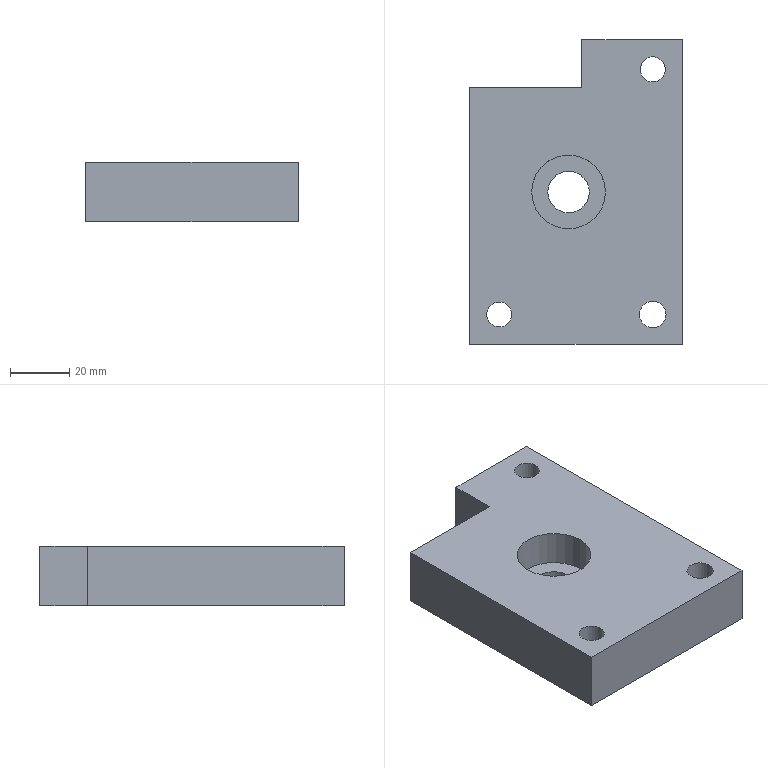Part | NX | features solid 2 | 1 solid | 20 faces | box 72 x 103 x 20 mm | volume 122631 mm3 | plane 12 | cylinder 8 | commonest cylinder face diameters 14 x3 8.5 x2 9 x1 14.1 x1 25 x1
STEP:
#1=CARTESIAN_POINT('',(121.25,98.5,20.));
#2=VERTEX_POINT('',#1);
#3=CARTESIAN_POINT('',(125.5,98.5,20.));
#4=DIRECTION('',(0.,0.,-1.));
#5=DIRECTION('',(-1.,0.,0.));
#6=AXIS2_PLACEMENT_3D('',#3,#4,#5);
#7=CIRCLE('',#6,4.25);
#8=EDGE_CURVE('',#2,#2,#7,.T.);
#9=ORIENTED_EDGE('',*,*,#8,.F.);
#10=EDGE_LOOP('',(#9));
#11=FACE_BOUND('',#10,.T.);
#12=CARTESIAN_POINT('',(121.25,98.5,10.));
#13=VERTEX_POINT('',#12);
#14=CARTESIAN_POINT('',(125.5,98.5,10.));
#15=DIRECTION('',(0.,0.,-1.));
#16=DIRECTION('',(-1.,0.,0.));
#17=AXIS2_PLACEMENT_3D('',#14,#15,#16);
#18=CIRCLE('',#17,4.25);
#19=EDGE_CURVE('',#13,#13,#18,.T.);
#20=ORIENTED_EDGE('',*,*,#19,.T.);
#21=EDGE_LOOP('',(#20));
#22=FACE_BOUND('',#21,.T.);
#23=CARTESIAN_POINT('',(125.5,98.5,35.));
#24=DIRECTION('',(0.,0.,1.));
#25=DIRECTION('',(1.,0.,0.));
#26=AXIS2_PLACEMENT_3D('',#23,#24,#25);
#27=CYLINDRICAL_SURFACE('',#26,4.25);
#28=ADVANCED_FACE('',(#11,#22),#27,.F.);
#29=CARTESIAN_POINT('',(118.5,98.5,10.));
#30=VERTEX_POINT('',#29);
#31=CARTESIAN_POINT('',(125.5,98.5,10.));
#32=DIRECTION('',(0.,0.,-1.));
#33=DIRECTION('',(-1.,0.,0.));
#34=AXIS2_PLACEMENT_3D('',#31,#32,#33);
#35=CIRCLE('',#34,7.);
#36=EDGE_CURVE('',#30,#30,#35,.T.);
#37=ORIENTED_EDGE('',*,*,#36,.F.);
#38=EDGE_LOOP('',(#37));
#39=FACE_BOUND('',#38,.T.);
#40=CARTESIAN_POINT('',(132.5,98.5,0.00000121));
#41=VERTEX_POINT('',#40);
#42=CARTESIAN_POINT('',(125.5,98.5,0.00000121));
#43=DIRECTION('',(0.,0.,1.));
#44=DIRECTION('',(1.,0.,0.));
#45=AXIS2_PLACEMENT_3D('',#42,#43,#44);
#46=CIRCLE('',#45,7.);
#47=EDGE_CURVE('',#41,#41,#46,.T.);
#48=ORIENTED_EDGE('',*,*,#47,.F.);
#49=EDGE_LOOP('',(#48));
#50=FACE_BOUND('',#49,.T.);
#51=CARTESIAN_POINT('',(125.5,98.5,0.00000121));
#52=DIRECTION('',(0.,0.,1.));
#53=DIRECTION('',(1.,0.,0.));
#54=AXIS2_PLACEMENT_3D('',#51,#52,#53);
#55=CYLINDRICAL_SURFACE('',#54,7.);
#56=ADVANCED_FACE('',(#39,#50),#55,.F.);
#57=ORIENTED_EDGE('',*,*,#19,.F.);
#58=EDGE_LOOP('',(#57));
#59=FACE_BOUND('',#58,.T.);
#60=ORIENTED_EDGE('',*,*,#36,.T.);
#61=EDGE_LOOP('',(#60));
#62=FACE_BOUND('',#61,.T.);
#63=CARTESIAN_POINT('',(11.595,84.569,10.));
#64=DIRECTION('',(0.,0.,1.));
#65=DIRECTION('',(-1.,0.,0.));
#66=AXIS2_PLACEMENT_3D('',#63,#64,#65);
#67=PLANE('',#66);
#68=ADVANCED_FACE('',(#59,#62),#67,.F.);
#69=CARTESIAN_POINT('',(182.,98.5,10.));
#70=VERTEX_POINT('',#69);
#71=CARTESIAN_POINT('',(177.5,98.5,10.));
#72=DIRECTION('',(0.,0.,1.));
#73=DIRECTION('',(1.,0.,0.));
#74=AXIS2_PLACEMENT_3D('',#71,#72,#73);
#75=CIRCLE('',#74,4.5);
#76=EDGE_CURVE('',#70,#70,#75,.F.);
#77=ORIENTED_EDGE('',*,*,#76,.F.);
#78=EDGE_LOOP('',(#77));
#79=FACE_BOUND('',#78,.T.);
#80=CARTESIAN_POINT('',(184.5,98.5,10.));
#81=VERTEX_POINT('',#80);
#82=CARTESIAN_POINT('',(177.5,98.5,10.));
#83=DIRECTION('',(0.,0.,1.));
#84=DIRECTION('',(1.,0.,0.));
#85=AXIS2_PLACEMENT_3D('',#82,#83,#84);
#86=CIRCLE('',#85,7.);
#87=EDGE_CURVE('',#81,#81,#86,.F.);
#88=ORIENTED_EDGE('',*,*,#87,.T.);
#89=EDGE_LOOP('',(#88));
#90=FACE_BOUND('',#89,.T.);
#91=CARTESIAN_POINT('',(291.405,84.569,10.));
#92=DIRECTION('',(0.,0.,1.));
#93=DIRECTION('',(1.,0.,0.));
#94=AXIS2_PLACEMENT_3D('',#91,#92,#93);
#95=PLANE('',#94);
#96=ADVANCED_FACE('',(#79,#90),#95,.F.);
#97=CARTESIAN_POINT('',(181.75,181.5,10.));
#98=VERTEX_POINT('',#97);
#99=CARTESIAN_POINT('',(177.5,181.5,10.));
#100=DIRECTION('',(0.,0.,-1.));
#101=DIRECTION('',(1.,0.,0.));
#102=AXIS2_PLACEMENT_3D('',#99,#100,#101);
#103=CIRCLE('',#102,4.25);
#104=EDGE_CURVE('',#98,#98,#103,.T.);
#105=ORIENTED_EDGE('',*,*,#104,.F.);
#106=EDGE_LOOP('',(#105));
#107=FACE_BOUND('',#106,.T.);
#108=CARTESIAN_POINT('',(184.5,181.5,10.));
#109=VERTEX_POINT('',#108);
#110=CARTESIAN_POINT('',(177.5,181.5,10.));
#111=DIRECTION('',(0.,0.,-1.));
#112=DIRECTION('',(1.,0.,0.));
#113=AXIS2_PLACEMENT_3D('',#110,#111,#112);
#114=CIRCLE('',#113,7.);
#115=EDGE_CURVE('',#109,#109,#114,.T.);
#116=ORIENTED_EDGE('',*,*,#115,.T.);
#117=EDGE_LOOP('',(#116));
#118=FACE_BOUND('',#117,.T.);
#119=CARTESIAN_POINT('',(291.405,195.431,10.));
#120=DIRECTION('',(0.,0.,1.));
#121=DIRECTION('',(1.,0.,0.));
#122=AXIS2_PLACEMENT_3D('',#119,#120,#121);
#123=PLANE('',#122);
#124=ADVANCED_FACE('',(#107,#118),#123,.F.);
#125=ORIENTED_EDGE('',*,*,#87,.F.);
#126=EDGE_LOOP('',(#125));
#127=FACE_BOUND('',#126,.T.);
#128=CARTESIAN_POINT('',(170.5,98.5,0.00000121));
#129=VERTEX_POINT('',#128);
#130=CARTESIAN_POINT('',(177.5,98.5,0.00000121));
#131=DIRECTION('',(0.,0.,-1.));
#132=DIRECTION('',(-1.,0.,0.));
#133=AXIS2_PLACEMENT_3D('',#130,#131,#132);
#134=CIRCLE('',#133,7.);
#135=EDGE_CURVE('',#129,#129,#134,.F.);
#136=ORIENTED_EDGE('',*,*,#135,.F.);
#137=EDGE_LOOP('',(#136));
#138=FACE_BOUND('',#137,.T.);
#139=CARTESIAN_POINT('',(177.5,98.5,0.00000121));
#140=DIRECTION('',(0.,0.,1.));
#141=DIRECTION('',(-1.,0.,0.));
#142=AXIS2_PLACEMENT_3D('',#139,#140,#141);
#143=CYLINDRICAL_SURFACE('',#142,7.);
#144=ADVANCED_FACE('',(#127,#138),#143,.F.);
#145=ORIENTED_EDGE('',*,*,#115,.F.);
#146=EDGE_LOOP('',(#145));
#147=FACE_BOUND('',#146,.T.);
#148=CARTESIAN_POINT('',(170.5,181.5,0.00000121));
#149=VERTEX_POINT('',#148);
#150=CARTESIAN_POINT('',(177.5,181.5,0.00000121));
#151=DIRECTION('',(0.,0.,1.));
#152=DIRECTION('',(-1.,0.,0.));
#153=AXIS2_PLACEMENT_3D('',#150,#151,#152);
#154=CIRCLE('',#153,7.);
#155=EDGE_CURVE('',#149,#149,#154,.T.);
#156=ORIENTED_EDGE('',*,*,#155,.F.);
#157=EDGE_LOOP('',(#156));
#158=FACE_BOUND('',#157,.T.);
#159=CARTESIAN_POINT('',(177.5,181.5,0.00000121));
#160=DIRECTION('',(0.,0.,1.));
#161=DIRECTION('',(-1.,0.,0.));
#162=AXIS2_PLACEMENT_3D('',#159,#160,#161);
#163=CYLINDRICAL_SURFACE('',#162,7.);
#164=ADVANCED_FACE('',(#147,#158),#163,.F.);
#165=CARTESIAN_POINT('',(161.5,140.,8.));
#166=VERTEX_POINT('',#165);
#167=CARTESIAN_POINT('',(149.,140.,8.));
#168=DIRECTION('',(0.,0.,1.));
#169=DIRECTION('',(1.,0.,0.));
#170=AXIS2_PLACEMENT_3D('',#167,#168,#169);
#171=CIRCLE('',#170,12.5);
#172=EDGE_CURVE('',#166,#166,#171,.F.);
#173=ORIENTED_EDGE('',*,*,#172,.T.);
#174=EDGE_LOOP('',(#173));
#175=FACE_BOUND('',#174,.T.);
#176=CARTESIAN_POINT('',(161.5,140.,20.));
#177=VERTEX_POINT('',#176);
#178=CARTESIAN_POINT('',(149.,140.,20.));
#179=DIRECTION('',(0.,0.,1.));
#180=DIRECTION('',(1.,0.,0.));
#181=AXIS2_PLACEMENT_3D('',#178,#179,#180);
#182=CIRCLE('',#181,12.5);
#183=EDGE_CURVE('',#177,#177,#182,.F.);
#184=ORIENTED_EDGE('',*,*,#183,.F.);
#185=EDGE_LOOP('',(#184));
#186=FACE_BOUND('',#185,.T.);
#187=CARTESIAN_POINT('',(149.,140.,2.5));
#188=DIRECTION('',(0.,0.,-1.));
#189=DIRECTION('',(-1.,0.,0.));
#190=AXIS2_PLACEMENT_3D('',#187,#188,#189);
#191=CYLINDRICAL_SURFACE('',#190,12.5);
#192=ADVANCED_FACE('',(#175,#186),#191,.F.);
#193=CARTESIAN_POINT('',(187.5,88.5,20.));
#194=VERTEX_POINT('',#193);
#195=CARTESIAN_POINT('',(187.5,88.5,0.00000121));
#196=VERTEX_POINT('',#195);
#197=CARTESIAN_POINT('',(187.5,88.5,35.));
#198=DIRECTION('',(0.,0.,-1.));
#199=VECTOR('',#198,1000.);
#200=LINE('',#197,#199);
#201=EDGE_CURVE('',#194,#196,#200,.T.);
#202=ORIENTED_EDGE('',*,*,#201,.T.);
#203=CARTESIAN_POINT('',(187.5,191.5,0.00000121));
#204=VERTEX_POINT('',#203);
#205=CARTESIAN_POINT('',(187.5,140.,0.00000121));
#206=DIRECTION('',(0.,-1.,0.));
#207=VECTOR('',#206,1000.);
#208=LINE('',#205,#207);
#209=EDGE_CURVE('',#196,#204,#208,.F.);
#210=ORIENTED_EDGE('',*,*,#209,.T.);
#211=CARTESIAN_POINT('',(187.5,191.5,20.));
#212=VERTEX_POINT('',#211);
#213=CARTESIAN_POINT('',(187.5,191.5,35.));
#214=DIRECTION('',(0.,0.,-1.));
#215=VECTOR('',#214,1000.);
#216=LINE('',#213,#215);
#217=EDGE_CURVE('',#212,#204,#216,.T.);
#218=ORIENTED_EDGE('',*,*,#217,.F.);
#219=CARTESIAN_POINT('',(187.5,140.,20.));
#220=DIRECTION('',(0.,1.,0.));
#221=VECTOR('',#220,1000.);
#222=LINE('',#219,#221);
#223=EDGE_CURVE('',#194,#212,#222,.T.);
#224=ORIENTED_EDGE('',*,*,#223,.F.);
#225=EDGE_LOOP('',(#202,#210,#218,#224));
#226=FACE_BOUND('',#225,.T.);
#227=CARTESIAN_POINT('',(187.5,140.,35.));
#228=DIRECTION('',(-1.,0.,0.));
#229=DIRECTION('',(0.,1.,0.));
#230=AXIS2_PLACEMENT_3D('',#227,#228,#229);
#231=PLANE('',#230);
#232=ADVANCED_FACE('',(#226),#231,.F.);
#233=CARTESIAN_POINT('',(115.5,88.5,20.));
#234=VERTEX_POINT('',#233);
#235=CARTESIAN_POINT('',(115.5,88.5,0.00000121));
#236=VERTEX_POINT('',#235);
#237=CARTESIAN_POINT('',(115.5,88.5,35.));
#238=DIRECTION('',(0.,0.,-1.));
#239=VECTOR('',#238,1000.);
#240=LINE('',#237,#239);
#241=EDGE_CURVE('',#234,#236,#240,.T.);
#242=ORIENTED_EDGE('',*,*,#241,.T.);
#243=CARTESIAN_POINT('',(149.,88.5,0.00000121));
#244=DIRECTION('',(-1.,0.,0.));
#245=VECTOR('',#244,1000.);
#246=LINE('',#243,#245);
#247=EDGE_CURVE('',#236,#196,#246,.F.);
#248=ORIENTED_EDGE('',*,*,#247,.T.);
#249=ORIENTED_EDGE('',*,*,#201,.F.);
#250=CARTESIAN_POINT('',(149.,88.5,20.));
#251=DIRECTION('',(1.,0.,0.));
#252=VECTOR('',#251,1000.);
#253=LINE('',#250,#252);
#254=EDGE_CURVE('',#234,#194,#253,.T.);
#255=ORIENTED_EDGE('',*,*,#254,.F.);
#256=EDGE_LOOP('',(#242,#248,#249,#255));
#257=FACE_BOUND('',#256,.T.);
#258=CARTESIAN_POINT('',(149.,88.5,35.));
#259=DIRECTION('',(0.,1.,0.));
#260=DIRECTION('',(1.,0.,0.));
#261=AXIS2_PLACEMENT_3D('',#258,#259,#260);
#262=PLANE('',#261);
#263=ADVANCED_FACE('',(#257),#262,.F.);
#264=CARTESIAN_POINT('',(115.5,175.5,0.00000121));
#265=VERTEX_POINT('',#264);
#266=CARTESIAN_POINT('',(115.5,175.5,20.));
#267=VERTEX_POINT('',#266);
#268=CARTESIAN_POINT('',(115.5,175.5,35.));
#269=DIRECTION('',(0.,0.,1.));
#270=VECTOR('',#269,1000.);
#271=LINE('',#268,#270);
#272=EDGE_CURVE('',#265,#267,#271,.T.);
#273=ORIENTED_EDGE('',*,*,#272,.F.);
#274=CARTESIAN_POINT('',(115.5,140.,0.00000121));
#275=DIRECTION('',(0.,1.,0.));
#276=VECTOR('',#275,1000.);
#277=LINE('',#274,#276);
#278=EDGE_CURVE('',#265,#236,#277,.F.);
#279=ORIENTED_EDGE('',*,*,#278,.T.);
#280=ORIENTED_EDGE('',*,*,#241,.F.);
#281=CARTESIAN_POINT('',(115.5,140.,20.));
#282=DIRECTION('',(0.,-1.,0.));
#283=VECTOR('',#282,1000.);
#284=LINE('',#281,#283);
#285=EDGE_CURVE('',#267,#234,#284,.T.);
#286=ORIENTED_EDGE('',*,*,#285,.F.);
#287=EDGE_LOOP('',(#273,#279,#280,#286));
#288=FACE_BOUND('',#287,.T.);
#289=CARTESIAN_POINT('',(115.5,140.,35.));
#290=DIRECTION('',(1.,0.,0.));
#291=DIRECTION('',(0.,-1.,0.));
#292=AXIS2_PLACEMENT_3D('',#289,#290,#291);
#293=PLANE('',#292);
#294=ADVANCED_FACE('',(#288),#293,.F.);
#295=CARTESIAN_POINT('',(153.5,175.5,20.));
#296=VERTEX_POINT('',#295);
#297=CARTESIAN_POINT('',(153.5,175.5,0.00000121));
#298=VERTEX_POINT('',#297);
#299=CARTESIAN_POINT('',(153.5,175.5,-10.));
#300=DIRECTION('',(0.,0.,1.));
#301=VECTOR('',#300,1000.);
#302=LINE('',#299,#301);
#303=EDGE_CURVE('',#296,#298,#302,.F.);
#304=ORIENTED_EDGE('',*,*,#303,.T.);
#305=CARTESIAN_POINT('',(149.,175.5,0.00000121));
#306=DIRECTION('',(1.,0.,0.));
#307=VECTOR('',#306,1000.);
#308=LINE('',#305,#307);
#309=EDGE_CURVE('',#298,#265,#308,.F.);
#310=ORIENTED_EDGE('',*,*,#309,.T.);
#311=ORIENTED_EDGE('',*,*,#272,.T.);
#312=CARTESIAN_POINT('',(251.29,175.5,20.));
#313=DIRECTION('',(-1.,0.,0.));
#314=VECTOR('',#313,1000.);
#315=LINE('',#312,#314);
#316=EDGE_CURVE('',#296,#267,#315,.T.);
#317=ORIENTED_EDGE('',*,*,#316,.F.);
#318=EDGE_LOOP('',(#304,#310,#311,#317));
#319=FACE_BOUND('',#318,.T.);
#320=CARTESIAN_POINT('',(149.,175.5,42.));
#321=DIRECTION('',(0.,1.,0.));
#322=DIRECTION('',(-1.,0.,0.));
#323=AXIS2_PLACEMENT_3D('',#320,#321,#322);
#324=PLANE('',#323);
#325=ADVANCED_FACE('',(#319),#324,.T.);
#326=CARTESIAN_POINT('',(153.5,191.5,20.));
#327=VERTEX_POINT('',#326);
#328=CARTESIAN_POINT('',(153.5,191.5,0.00000121));
#329=VERTEX_POINT('',#328);
#330=CARTESIAN_POINT('',(153.5,191.5,35.));
#331=DIRECTION('',(0.,0.,1.));
#332=VECTOR('',#331,1000.);
#333=LINE('',#330,#332);
#334=EDGE_CURVE('',#327,#329,#333,.F.);
#335=ORIENTED_EDGE('',*,*,#334,.T.);
#336=CARTESIAN_POINT('',(153.5,140.,0.00000121));
#337=DIRECTION('',(0.,-1.,0.));
#338=VECTOR('',#337,1000.);
#339=LINE('',#336,#338);
#340=EDGE_CURVE('',#329,#298,#339,.T.);
#341=ORIENTED_EDGE('',*,*,#340,.T.);
#342=ORIENTED_EDGE('',*,*,#303,.F.);
#343=CARTESIAN_POINT('',(153.5,25.984,20.));
#344=DIRECTION('',(0.,1.,0.));
#345=VECTOR('',#344,1000.);
#346=LINE('',#343,#345);
#347=EDGE_CURVE('',#327,#296,#346,.F.);
#348=ORIENTED_EDGE('',*,*,#347,.F.);
#349=EDGE_LOOP('',(#335,#341,#342,#348));
#350=FACE_BOUND('',#349,.T.);
#351=CARTESIAN_POINT('',(153.5,183.,-10.));
#352=DIRECTION('',(1.,0.,0.));
#353=DIRECTION('',(0.,1.,0.));
#354=AXIS2_PLACEMENT_3D('',#351,#352,#353);
#355=PLANE('',#354);
#356=ADVANCED_FACE('',(#350),#355,.F.);
#357=ORIENTED_EDGE('',*,*,#217,.T.);
#358=CARTESIAN_POINT('',(149.,191.5,0.00000121));
#359=DIRECTION('',(1.,0.,0.));
#360=VECTOR('',#359,1000.);
#361=LINE('',#358,#360);
#362=EDGE_CURVE('',#204,#329,#361,.F.);
#363=ORIENTED_EDGE('',*,*,#362,.T.);
#364=ORIENTED_EDGE('',*,*,#334,.F.);
#365=CARTESIAN_POINT('',(149.,191.5,20.));
#366=DIRECTION('',(-1.,0.,0.));
#367=VECTOR('',#366,1000.);
#368=LINE('',#365,#367);
#369=EDGE_CURVE('',#212,#327,#368,.T.);
#370=ORIENTED_EDGE('',*,*,#369,.F.);
#371=EDGE_LOOP('',(#357,#363,#364,#370));
#372=FACE_BOUND('',#371,.T.);
#373=CARTESIAN_POINT('',(149.,191.5,35.));
#374=DIRECTION('',(0.,-1.,0.));
#375=DIRECTION('',(-1.,0.,0.));
#376=AXIS2_PLACEMENT_3D('',#373,#374,#375);
#377=PLANE('',#376);
#378=ADVANCED_FACE('',(#372),#377,.F.);
#379=CARTESIAN_POINT('',(182.,98.5,20.));
#380=VERTEX_POINT('',#379);
#381=CARTESIAN_POINT('',(177.5,98.5,20.));
#382=DIRECTION('',(0.,0.,1.));
#383=DIRECTION('',(1.,0.,0.));
#384=AXIS2_PLACEMENT_3D('',#381,#382,#383);
#385=CIRCLE('',#384,4.5);
#386=EDGE_CURVE('',#380,#380,#385,.F.);
#387=ORIENTED_EDGE('',*,*,#386,.F.);
#388=EDGE_LOOP('',(#387));
#389=FACE_BOUND('',#388,.T.);
#390=ORIENTED_EDGE('',*,*,#76,.T.);
#391=EDGE_LOOP('',(#390));
#392=FACE_BOUND('',#391,.T.);
#393=CARTESIAN_POINT('',(177.5,98.5,35.));
#394=DIRECTION('',(0.,0.,1.));
#395=DIRECTION('',(-1.,0.,0.));
#396=AXIS2_PLACEMENT_3D('',#393,#394,#395);
#397=CYLINDRICAL_SURFACE('',#396,4.5);
#398=ADVANCED_FACE('',(#389,#392),#397,.F.);
#399=CARTESIAN_POINT('',(181.75,181.5,20.));
#400=VERTEX_POINT('',#399);
#401=CARTESIAN_POINT('',(177.5,181.5,20.));
#402=DIRECTION('',(0.,0.,-1.));
#403=DIRECTION('',(1.,0.,0.));
#404=AXIS2_PLACEMENT_3D('',#401,#402,#403);
#405=CIRCLE('',#404,4.25);
#406=EDGE_CURVE('',#400,#400,#405,.T.);
#407=ORIENTED_EDGE('',*,*,#406,.F.);
#408=EDGE_LOOP('',(#407));
#409=FACE_BOUND('',#408,.T.);
#410=ORIENTED_EDGE('',*,*,#104,.T.);
#411=EDGE_LOOP('',(#410));
#412=FACE_BOUND('',#411,.T.);
#413=CARTESIAN_POINT('',(177.5,181.5,35.));
#414=DIRECTION('',(0.,0.,1.));
#415=DIRECTION('',(-1.,0.,0.));
#416=AXIS2_PLACEMENT_3D('',#413,#414,#415);
#417=CYLINDRICAL_SURFACE('',#416,4.25);
#418=ADVANCED_FACE('',(#409,#412),#417,.F.);
#419=ORIENTED_EDGE('',*,*,#8,.T.);
#420=EDGE_LOOP('',(#419));
#421=FACE_BOUND('',#420,.T.);
#422=ORIENTED_EDGE('',*,*,#406,.T.);
#423=EDGE_LOOP('',(#422));
#424=FACE_BOUND('',#423,.T.);
#425=ORIENTED_EDGE('',*,*,#386,.T.);
#426=EDGE_LOOP('',(#425));
#427=FACE_BOUND('',#426,.T.);
#428=ORIENTED_EDGE('',*,*,#369,.T.);
#429=ORIENTED_EDGE('',*,*,#347,.T.);
#430=ORIENTED_EDGE('',*,*,#316,.T.);
#431=ORIENTED_EDGE('',*,*,#285,.T.);
#432=ORIENTED_EDGE('',*,*,#254,.T.);
#433=ORIENTED_EDGE('',*,*,#223,.T.);
#434=EDGE_LOOP('',(#428,#429,#430,#431,#432,#433));
#435=FACE_BOUND('',#434,.T.);
#436=ORIENTED_EDGE('',*,*,#183,.T.);
#437=EDGE_LOOP('',(#436));
#438=FACE_BOUND('',#437,.T.);
#439=CARTESIAN_POINT('',(251.29,25.984,20.));
#440=DIRECTION('',(0.,0.,1.));
#441=DIRECTION('',(1.,0.,0.));
#442=AXIS2_PLACEMENT_3D('',#439,#440,#441);
#443=PLANE('',#442);
#444=ADVANCED_FACE('',(#421,#424,#427,#435,#438),#443,.T.);
#445=CARTESIAN_POINT('',(156.05,140.,8.));
#446=VERTEX_POINT('',#445);
#447=CARTESIAN_POINT('',(149.,140.,8.));
#448=DIRECTION('',(0.,0.,1.));
#449=DIRECTION('',(1.,0.,0.));
#450=AXIS2_PLACEMENT_3D('',#447,#448,#449);
#451=CIRCLE('',#450,7.05);
#452=EDGE_CURVE('',#446,#446,#451,.T.);
#453=ORIENTED_EDGE('',*,*,#452,.F.);
#454=EDGE_LOOP('',(#453));
#455=FACE_BOUND('',#454,.T.);
#456=ORIENTED_EDGE('',*,*,#172,.F.);
#457=EDGE_LOOP('',(#456));
#458=FACE_BOUND('',#457,.T.);
#459=CARTESIAN_POINT('',(151.5,140.,8.));
#460=DIRECTION('',(0.,0.,1.));
#461=DIRECTION('',(1.,0.,0.));
#462=AXIS2_PLACEMENT_3D('',#459,#460,#461);
#463=PLANE('',#462);
#464=ADVANCED_FACE('',(#455,#458),#463,.T.);
#465=CARTESIAN_POINT('',(141.95,140.,0.00000121));
#466=VERTEX_POINT('',#465);
#467=CARTESIAN_POINT('',(149.,140.,0.00000121));
#468=DIRECTION('',(0.,0.,-1.));
#469=DIRECTION('',(-1.,0.,0.));
#470=AXIS2_PLACEMENT_3D('',#467,#468,#469);
#471=CIRCLE('',#470,7.05);
#472=EDGE_CURVE('',#466,#466,#471,.F.);
#473=ORIENTED_EDGE('',*,*,#472,.F.);
#474=EDGE_LOOP('',(#473));
#475=FACE_BOUND('',#474,.T.);
#476=ORIENTED_EDGE('',*,*,#452,.T.);
#477=EDGE_LOOP('',(#476));
#478=FACE_BOUND('',#477,.T.);
#479=CARTESIAN_POINT('',(149.,140.,2.5));
#480=DIRECTION('',(0.,0.,-1.));
#481=DIRECTION('',(-1.,0.,0.));
#482=AXIS2_PLACEMENT_3D('',#479,#480,#481);
#483=CYLINDRICAL_SURFACE('',#482,7.05);
#484=ADVANCED_FACE('',(#475,#478),#483,.F.);
#485=ORIENTED_EDGE('',*,*,#47,.T.);
#486=EDGE_LOOP('',(#485));
#487=FACE_BOUND('',#486,.T.);
#488=ORIENTED_EDGE('',*,*,#340,.F.);
#489=ORIENTED_EDGE('',*,*,#362,.F.);
#490=ORIENTED_EDGE('',*,*,#209,.F.);
#491=ORIENTED_EDGE('',*,*,#247,.F.);
#492=ORIENTED_EDGE('',*,*,#278,.F.);
#493=ORIENTED_EDGE('',*,*,#309,.F.);
#494=EDGE_LOOP('',(#488,#489,#490,#491,#492,#493));
#495=FACE_BOUND('',#494,.T.);
#496=ORIENTED_EDGE('',*,*,#155,.T.);
#497=EDGE_LOOP('',(#496));
#498=FACE_BOUND('',#497,.T.);
#499=ORIENTED_EDGE('',*,*,#472,.T.);
#500=EDGE_LOOP('',(#499));
#501=FACE_BOUND('',#500,.T.);
#502=ORIENTED_EDGE('',*,*,#135,.T.);
#503=EDGE_LOOP('',(#502));
#504=FACE_BOUND('',#503,.T.);
#505=CARTESIAN_POINT('',(149.,140.,0.00000121));
#506=DIRECTION('',(0.,0.,-1.));
#507=DIRECTION('',(-1.,0.,0.));
#508=AXIS2_PLACEMENT_3D('',#505,#506,#507);
#509=PLANE('',#508);
#510=ADVANCED_FACE('',(#487,#495,#498,#501,#504),#509,.T.);
#511=CLOSED_SHELL('',(#28,#56,#68,#96,#124,#144,#164,#192,#232,#263,#294,#325,#356,#378,#398,#418,#444,#464,#484,#510));
#512=MANIFOLD_SOLID_BREP('',#511);
#513=(LENGTH_UNIT()NAMED_UNIT(*)SI_UNIT(.MILLI.,.METRE.));
#514=UNCERTAINTY_MEASURE_WITH_UNIT(LENGTH_MEASURE(0.00001),#513,'','');
#515=(NAMED_UNIT(*)PLANE_ANGLE_UNIT()SI_UNIT($,.RADIAN.));
#516=(NAMED_UNIT(*)SI_UNIT($,.STERADIAN.)SOLID_ANGLE_UNIT());
#517=(GEOMETRIC_REPRESENTATION_CONTEXT(3)GLOBAL_UNCERTAINTY_ASSIGNED_CONTEXT((#514))GLOBAL_UNIT_ASSIGNED_CONTEXT((#513,#515,#516))REPRESENTATION_CONTEXT('',''));
#518=ADVANCED_BREP_SHAPE_REPRESENTATION('',(#512),#517);